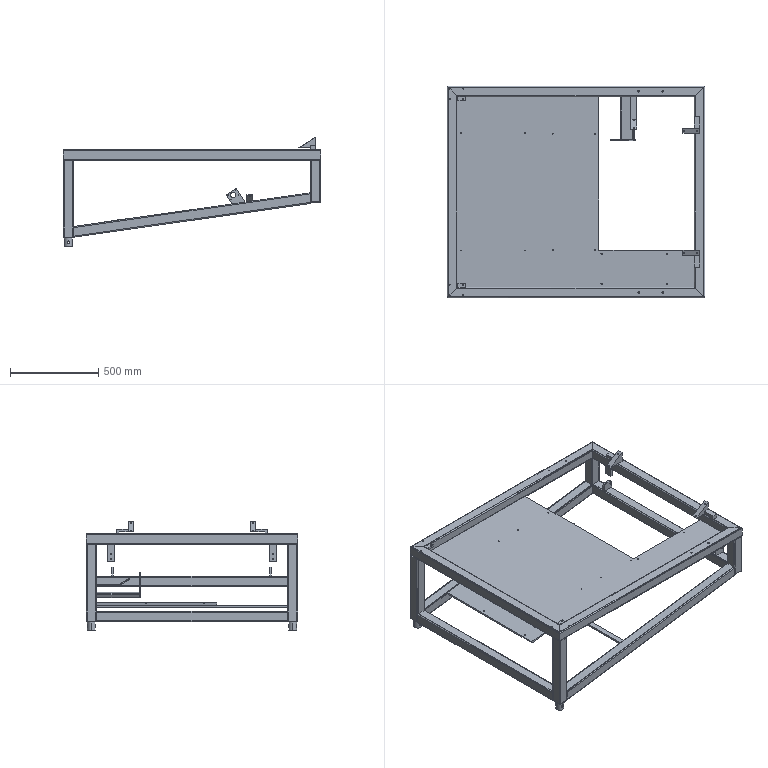Part | SolidWorks | features ICE 14, MoveCopyBody 6, WeldMemberFeat 4, Fillet 3, HoleWzd 3, BossThin 2, Cut 2, EndCap 2, MirrorSolid 2, WeldCornerFeat 2, WeldmentFeature 1 | 32 solids | 487 faces | box 1460 x 1200 x 621.009 mm | volume 23985037 mm3 | plane 246 | cylinder 237 | cone 4 | commonest cylinder face diameters 12 x53 2 x48 6.8 x26 7 x20 5 x16 6 x16